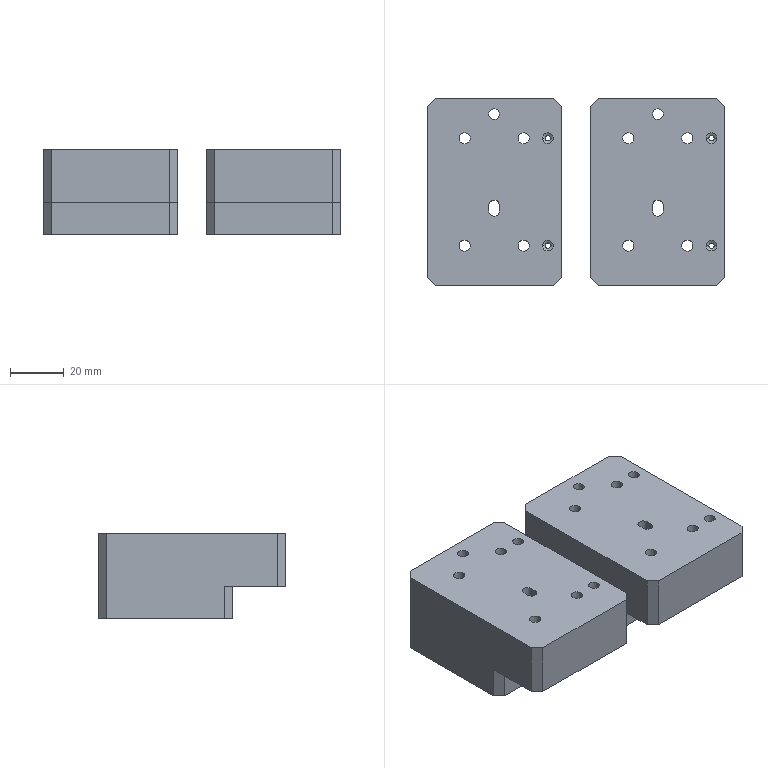NC program | NX | posted with a generic post | part box 111 x 70 x 32 mm
Lines 1 to 18 of 5357:
N10 G17 G21 G94 G90
(FLOOR_WALL , TOOL : D80)
N12 T19 M6
N14 G54
N16 G17 G0 G90 X-45. Y35. S6500 M3
N18 G43 Z30. H19
N20 Z3.
N22 G94 G1 Z0. F1500.
N24 X-42.
N26 X153.
N28 X156.
N30 Z3.
N32 G0 Z30.
N34 M5